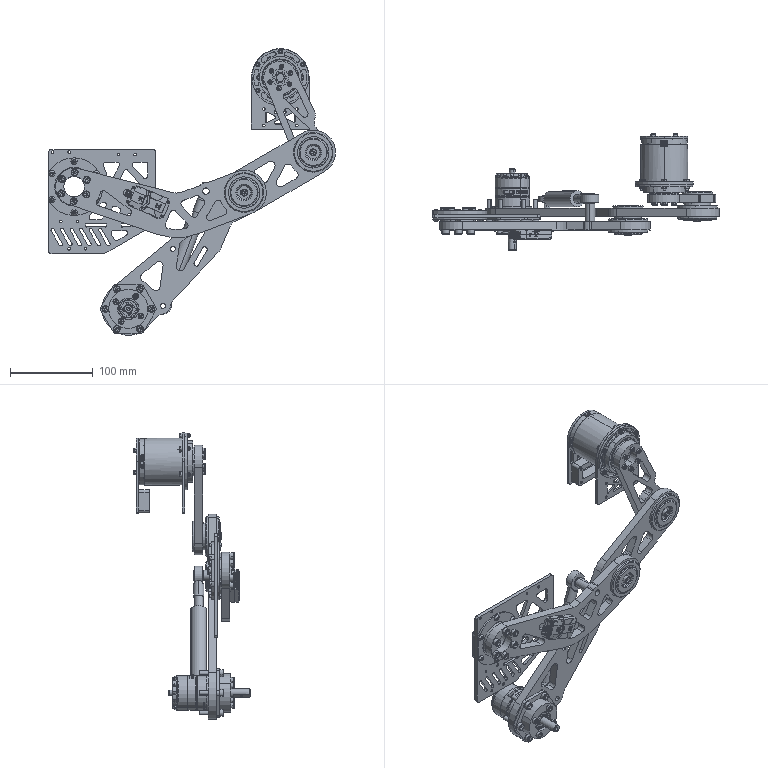Part | SolidWorks | features CompositeCurve 1 | 169 solids | 7589 faces | volume 699438 mm3 | plane 3501 | cylinder 2396 | spline 698 | cone 584 | torus 258 | sphere 152 | commonest cylinder face diameters 4 x204 0.2 x118 5 x105 2.5 x104 3.2 x104 6 x102